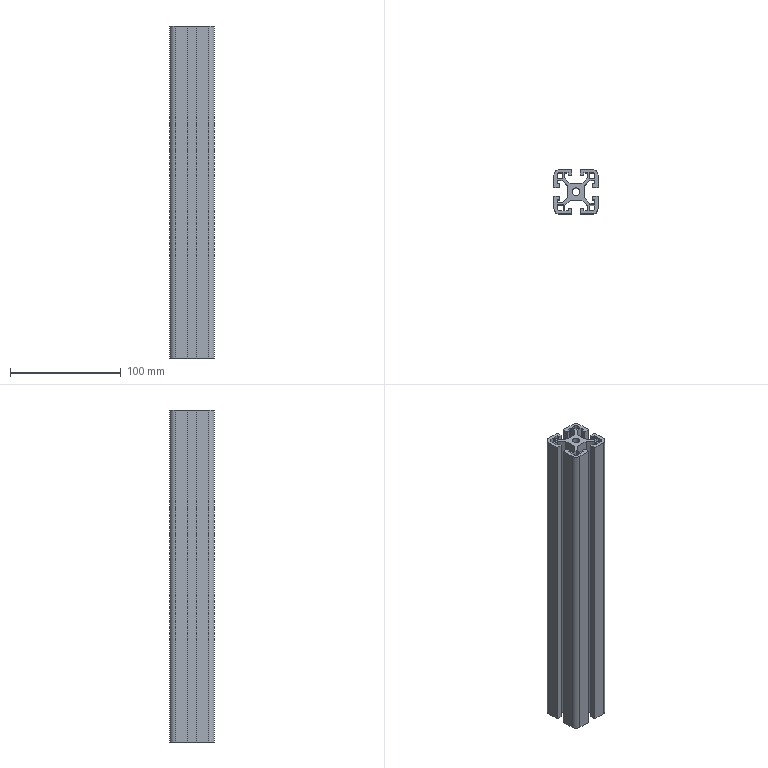Part | STEP file | 40x40-300 | 1 solid | 88 faces | box 40 x 40 x 300 mm | volume 211184 mm3 | plane 78 | cylinder 10 | commonest cylinder face diameters 4 x4 10 x4 6.8 x2